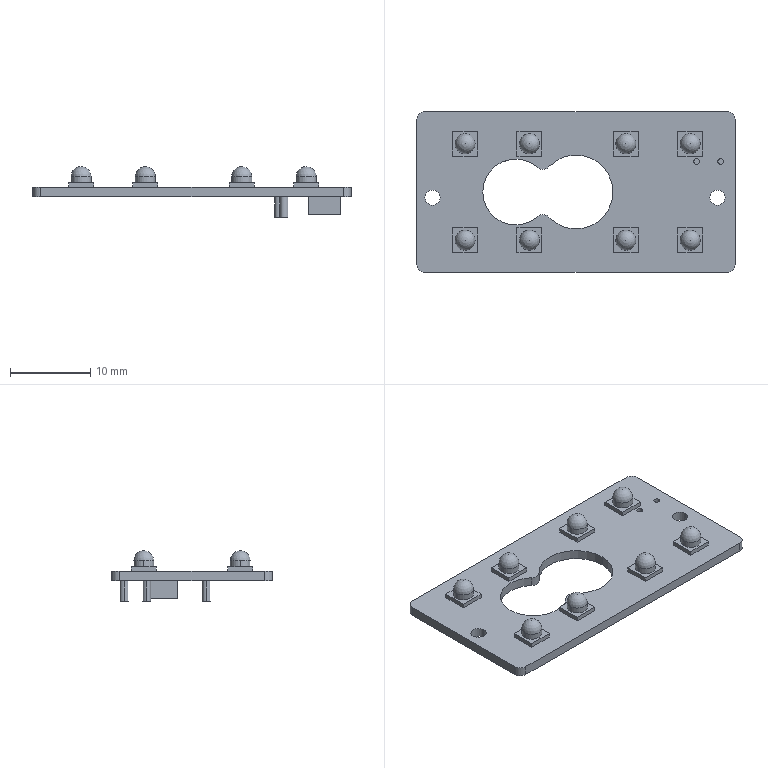Part | SolidWorks | features BaseBody 1 | 1 solid | 104 faces | box 39.6 x 20 x 6.29 mm | volume 948.766 mm3 | plane 56 | cylinder 40 | sphere 8 | commonest cylinder face diameters 2.5 x16 1.02 x6 2 x6 0.7 x4 1.9 x4 8.2 x2